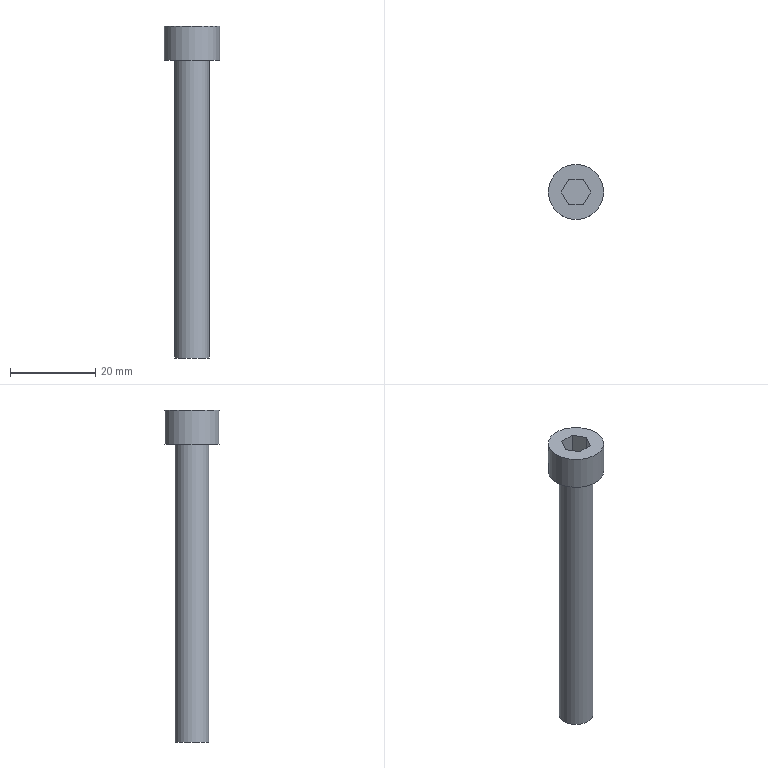Part | STEP file | 冲床-300配套压波_id198_x_t | 1 solid | 12 faces | box 13 x 13 x 78 mm | volume 4416 mm3 | plane 10 | cylinder 2 | commonest cylinder face diameters 8 x1 13 x1
STEP:
#1=CARTESIAN_POINT('',(1811.5,-85.,191.));
#2=VERTEX_POINT('',#1);
#3=CARTESIAN_POINT('',(1805.,-85.,191.));
#4=DIRECTION('',(0.,0.,1.));
#5=DIRECTION('',(1.,0.,0.));
#6=AXIS2_PLACEMENT_3D('',#3,#4,#5);
#7=CIRCLE('',#6,6.5);
#8=EDGE_CURVE('',#2,#2,#7,.T.);
#9=ORIENTED_EDGE('',*,*,#8,.T.);
#10=EDGE_LOOP('',(#9));
#11=FACE_BOUND('',#10,.T.);
#12=CARTESIAN_POINT('',(1803.268,-82.,191.));
#13=VERTEX_POINT('',#12);
#14=CARTESIAN_POINT('',(1806.732,-82.,191.));
#15=VERTEX_POINT('',#14);
#16=CARTESIAN_POINT('',(1803.268,-82.,191.));
#17=DIRECTION('',(1.,0.,0.));
#18=VECTOR('',#17,1.);
#19=LINE('',#16,#18);
#20=EDGE_CURVE('',#13,#15,#19,.T.);
#21=ORIENTED_EDGE('',*,*,#20,.T.);
#22=CARTESIAN_POINT('',(1808.464,-85.,191.));
#23=VERTEX_POINT('',#22);
#24=CARTESIAN_POINT('',(1806.732,-82.,191.));
#25=DIRECTION('',(0.5,-0.866,0.));
#26=VECTOR('',#25,1.);
#27=LINE('',#24,#26);
#28=EDGE_CURVE('',#15,#23,#27,.T.);
#29=ORIENTED_EDGE('',*,*,#28,.T.);
#30=CARTESIAN_POINT('',(1806.732,-88.,191.));
#31=VERTEX_POINT('',#30);
#32=CARTESIAN_POINT('',(1808.464,-85.,191.));
#33=DIRECTION('',(-0.5,-0.866,0.));
#34=VECTOR('',#33,1.);
#35=LINE('',#32,#34);
#36=EDGE_CURVE('',#23,#31,#35,.T.);
#37=ORIENTED_EDGE('',*,*,#36,.T.);
#38=CARTESIAN_POINT('',(1803.268,-88.,191.));
#39=VERTEX_POINT('',#38);
#40=CARTESIAN_POINT('',(1806.732,-88.,191.));
#41=DIRECTION('',(-1.,0.,0.));
#42=VECTOR('',#41,1.);
#43=LINE('',#40,#42);
#44=EDGE_CURVE('',#31,#39,#43,.T.);
#45=ORIENTED_EDGE('',*,*,#44,.T.);
#46=CARTESIAN_POINT('',(1801.536,-85.,191.));
#47=VERTEX_POINT('',#46);
#48=CARTESIAN_POINT('',(1803.268,-88.,191.));
#49=DIRECTION('',(-0.5,0.866,0.));
#50=VECTOR('',#49,1.);
#51=LINE('',#48,#50);
#52=EDGE_CURVE('',#39,#47,#51,.T.);
#53=ORIENTED_EDGE('',*,*,#52,.T.);
#54=CARTESIAN_POINT('',(1801.536,-85.,191.));
#55=DIRECTION('',(0.5,0.866,0.));
#56=VECTOR('',#55,1.);
#57=LINE('',#54,#56);
#58=EDGE_CURVE('',#47,#13,#57,.T.);
#59=ORIENTED_EDGE('',*,*,#58,.T.);
#60=EDGE_LOOP('',(#21,#29,#37,#45,#53,#59));
#61=FACE_BOUND('',#60,.T.);
#62=CARTESIAN_POINT('',(1811.5,-85.,191.));
#63=DIRECTION('',(0.,0.,-1.));
#64=DIRECTION('',(-1.,0.,0.));
#65=AXIS2_PLACEMENT_3D('',#62,#63,#64);
#66=PLANE('',#65);
#67=ADVANCED_FACE('',(#11,#61),#66,.F.);
#68=ORIENTED_EDGE('',*,*,#8,.F.);
#69=EDGE_LOOP('',(#68));
#70=FACE_BOUND('',#69,.T.);
#71=CARTESIAN_POINT('',(1811.5,-85.,183.));
#72=VERTEX_POINT('',#71);
#73=CARTESIAN_POINT('',(1805.,-85.,183.));
#74=DIRECTION('',(0.,0.,1.));
#75=DIRECTION('',(1.,0.,0.));
#76=AXIS2_PLACEMENT_3D('',#73,#74,#75);
#77=CIRCLE('',#76,6.5);
#78=EDGE_CURVE('',#72,#72,#77,.T.);
#79=ORIENTED_EDGE('',*,*,#78,.T.);
#80=EDGE_LOOP('',(#79));
#81=FACE_BOUND('',#80,.T.);
#82=CARTESIAN_POINT('',(1805.,-85.,184.1));
#83=DIRECTION('',(0.,0.,1.));
#84=DIRECTION('',(1.,0.,0.));
#85=AXIS2_PLACEMENT_3D('',#82,#83,#84);
#86=CYLINDRICAL_SURFACE('',#85,6.5);
#87=ADVANCED_FACE('',(#70,#81),#86,.T.);
#88=ORIENTED_EDGE('',*,*,#78,.F.);
#89=EDGE_LOOP('',(#88));
#90=FACE_BOUND('',#89,.T.);
#91=CARTESIAN_POINT('',(1809.,-85.,183.));
#92=VERTEX_POINT('',#91);
#93=CARTESIAN_POINT('',(1805.,-85.,183.));
#94=DIRECTION('',(0.,0.,1.));
#95=DIRECTION('',(1.,0.,0.));
#96=AXIS2_PLACEMENT_3D('',#93,#94,#95);
#97=CIRCLE('',#96,4.);
#98=EDGE_CURVE('',#92,#92,#97,.T.);
#99=ORIENTED_EDGE('',*,*,#98,.T.);
#100=EDGE_LOOP('',(#99));
#101=FACE_BOUND('',#100,.T.);
#102=CARTESIAN_POINT('',(1809.,-85.,183.));
#103=DIRECTION('',(0.,0.,1.));
#104=DIRECTION('',(1.,0.,0.));
#105=AXIS2_PLACEMENT_3D('',#102,#103,#104);
#106=PLANE('',#105);
#107=ADVANCED_FACE('',(#90,#101),#106,.F.);
#108=ORIENTED_EDGE('',*,*,#98,.F.);
#109=EDGE_LOOP('',(#108));
#110=FACE_BOUND('',#109,.T.);
#111=CARTESIAN_POINT('',(1809.,-85.,113.));
#112=VERTEX_POINT('',#111);
#113=CARTESIAN_POINT('',(1805.,-85.,113.));
#114=DIRECTION('',(0.,0.,1.));
#115=DIRECTION('',(1.,0.,0.));
#116=AXIS2_PLACEMENT_3D('',#113,#114,#115);
#117=CIRCLE('',#116,4.);
#118=EDGE_CURVE('',#112,#112,#117,.T.);
#119=ORIENTED_EDGE('',*,*,#118,.T.);
#120=EDGE_LOOP('',(#119));
#121=FACE_BOUND('',#120,.T.);
#122=CARTESIAN_POINT('',(1805.,-85.,184.1));
#123=DIRECTION('',(0.,0.,1.));
#124=DIRECTION('',(1.,0.,0.));
#125=AXIS2_PLACEMENT_3D('',#122,#123,#124);
#126=CYLINDRICAL_SURFACE('',#125,4.);
#127=ADVANCED_FACE('',(#110,#121),#126,.T.);
#128=ORIENTED_EDGE('',*,*,#118,.F.);
#129=EDGE_LOOP('',(#128));
#130=FACE_OUTER_BOUND('',#129,.T.);
#131=CARTESIAN_POINT('',(1805.,-85.,113.));
#132=DIRECTION('',(0.,0.,1.));
#133=DIRECTION('',(1.,0.,0.));
#134=AXIS2_PLACEMENT_3D('',#131,#132,#133);
#135=PLANE('',#134);
#136=ADVANCED_FACE('',(#130),#135,.F.);
#137=ORIENTED_EDGE('',*,*,#20,.F.);
#138=CARTESIAN_POINT('',(1803.268,-82.,185.72));
#139=VERTEX_POINT('',#138);
#140=CARTESIAN_POINT('',(1803.268,-82.,185.72));
#141=DIRECTION('',(0.,0.,-1.));
#142=VECTOR('',#141,1.);
#143=LINE('',#140,#142);
#144=EDGE_CURVE('',#13,#139,#143,.T.);
#145=ORIENTED_EDGE('',*,*,#144,.T.);
#146=CARTESIAN_POINT('',(1806.732,-82.,185.72));
#147=VERTEX_POINT('',#146);
#148=CARTESIAN_POINT('',(1803.268,-82.,185.72));
#149=DIRECTION('',(-1.,0.,0.));
#150=VECTOR('',#149,1.);
#151=LINE('',#148,#150);
#152=EDGE_CURVE('',#147,#139,#151,.T.);
#153=ORIENTED_EDGE('',*,*,#152,.F.);
#154=CARTESIAN_POINT('',(1806.732,-82.,185.72));
#155=DIRECTION('',(0.,0.,-1.));
#156=VECTOR('',#155,1.);
#157=LINE('',#154,#156);
#158=EDGE_CURVE('',#15,#147,#157,.T.);
#159=ORIENTED_EDGE('',*,*,#158,.F.);
#160=EDGE_LOOP('',(#137,#145,#153,#159));
#161=FACE_OUTER_BOUND('',#160,.T.);
#162=CARTESIAN_POINT('',(1803.268,-82.,185.72));
#163=DIRECTION('',(0.,-1.,0.));
#164=DIRECTION('',(1.,0.,0.));
#165=AXIS2_PLACEMENT_3D('',#162,#163,#164);
#166=PLANE('',#165);
#167=ADVANCED_FACE('',(#161),#166,.T.);
#168=ORIENTED_EDGE('',*,*,#28,.F.);
#169=ORIENTED_EDGE('',*,*,#158,.T.);
#170=CARTESIAN_POINT('',(1808.464,-85.,185.72));
#171=VERTEX_POINT('',#170);
#172=CARTESIAN_POINT('',(1806.732,-82.,185.72));
#173=DIRECTION('',(-0.5,0.866,0.));
#174=VECTOR('',#173,1.);
#175=LINE('',#172,#174);
#176=EDGE_CURVE('',#171,#147,#175,.T.);
#177=ORIENTED_EDGE('',*,*,#176,.F.);
#178=CARTESIAN_POINT('',(1808.464,-85.,185.72));
#179=DIRECTION('',(0.,0.,-1.));
#180=VECTOR('',#179,1.);
#181=LINE('',#178,#180);
#182=EDGE_CURVE('',#23,#171,#181,.T.);
#183=ORIENTED_EDGE('',*,*,#182,.F.);
#184=EDGE_LOOP('',(#168,#169,#177,#183));
#185=FACE_OUTER_BOUND('',#184,.T.);
#186=CARTESIAN_POINT('',(1806.732,-82.,185.72));
#187=DIRECTION('',(-0.866,-0.5,0.));
#188=DIRECTION('',(0.5,-0.866,0.));
#189=AXIS2_PLACEMENT_3D('',#186,#187,#188);
#190=PLANE('',#189);
#191=ADVANCED_FACE('',(#185),#190,.T.);
#192=ORIENTED_EDGE('',*,*,#36,.F.);
#193=ORIENTED_EDGE('',*,*,#182,.T.);
#194=CARTESIAN_POINT('',(1806.732,-88.,185.72));
#195=VERTEX_POINT('',#194);
#196=CARTESIAN_POINT('',(1808.464,-85.,185.72));
#197=DIRECTION('',(0.5,0.866,0.));
#198=VECTOR('',#197,1.);
#199=LINE('',#196,#198);
#200=EDGE_CURVE('',#195,#171,#199,.T.);
#201=ORIENTED_EDGE('',*,*,#200,.F.);
#202=CARTESIAN_POINT('',(1806.732,-88.,185.72));
#203=DIRECTION('',(0.,0.,-1.));
#204=VECTOR('',#203,1.);
#205=LINE('',#202,#204);
#206=EDGE_CURVE('',#31,#195,#205,.T.);
#207=ORIENTED_EDGE('',*,*,#206,.F.);
#208=EDGE_LOOP('',(#192,#193,#201,#207));
#209=FACE_OUTER_BOUND('',#208,.T.);
#210=CARTESIAN_POINT('',(1808.464,-85.,185.72));
#211=DIRECTION('',(-0.866,0.5,0.));
#212=DIRECTION('',(-0.5,-0.866,0.));
#213=AXIS2_PLACEMENT_3D('',#210,#211,#212);
#214=PLANE('',#213);
#215=ADVANCED_FACE('',(#209),#214,.T.);
#216=ORIENTED_EDGE('',*,*,#44,.F.);
#217=ORIENTED_EDGE('',*,*,#206,.T.);
#218=CARTESIAN_POINT('',(1803.268,-88.,185.72));
#219=VERTEX_POINT('',#218);
#220=CARTESIAN_POINT('',(1806.732,-88.,185.72));
#221=DIRECTION('',(1.,0.,0.));
#222=VECTOR('',#221,1.);
#223=LINE('',#220,#222);
#224=EDGE_CURVE('',#219,#195,#223,.T.);
#225=ORIENTED_EDGE('',*,*,#224,.F.);
#226=CARTESIAN_POINT('',(1803.268,-88.,185.72));
#227=DIRECTION('',(0.,0.,-1.));
#228=VECTOR('',#227,1.);
#229=LINE('',#226,#228);
#230=EDGE_CURVE('',#39,#219,#229,.T.);
#231=ORIENTED_EDGE('',*,*,#230,.F.);
#232=EDGE_LOOP('',(#216,#217,#225,#231));
#233=FACE_OUTER_BOUND('',#232,.T.);
#234=CARTESIAN_POINT('',(1806.732,-88.,185.72));
#235=DIRECTION('',(0.,1.,0.));
#236=DIRECTION('',(-1.,0.,0.));
#237=AXIS2_PLACEMENT_3D('',#234,#235,#236);
#238=PLANE('',#237);
#239=ADVANCED_FACE('',(#233),#238,.T.);
#240=ORIENTED_EDGE('',*,*,#52,.F.);
#241=ORIENTED_EDGE('',*,*,#230,.T.);
#242=CARTESIAN_POINT('',(1801.536,-85.,185.72));
#243=VERTEX_POINT('',#242);
#244=CARTESIAN_POINT('',(1803.268,-88.,185.72));
#245=DIRECTION('',(0.5,-0.866,0.));
#246=VECTOR('',#245,1.);
#247=LINE('',#244,#246);
#248=EDGE_CURVE('',#243,#219,#247,.T.);
#249=ORIENTED_EDGE('',*,*,#248,.F.);
#250=CARTESIAN_POINT('',(1801.536,-85.,185.72));
#251=DIRECTION('',(0.,0.,-1.));
#252=VECTOR('',#251,1.);
#253=LINE('',#250,#252);
#254=EDGE_CURVE('',#47,#243,#253,.T.);
#255=ORIENTED_EDGE('',*,*,#254,.F.);
#256=EDGE_LOOP('',(#240,#241,#249,#255));
#257=FACE_OUTER_BOUND('',#256,.T.);
#258=CARTESIAN_POINT('',(1803.268,-88.,185.72));
#259=DIRECTION('',(0.866,0.5,0.));
#260=DIRECTION('',(-0.5,0.866,0.));
#261=AXIS2_PLACEMENT_3D('',#258,#259,#260);
#262=PLANE('',#261);
#263=ADVANCED_FACE('',(#257),#262,.T.);
#264=ORIENTED_EDGE('',*,*,#58,.F.);
#265=ORIENTED_EDGE('',*,*,#254,.T.);
#266=CARTESIAN_POINT('',(1801.536,-85.,185.72));
#267=DIRECTION('',(-0.5,-0.866,0.));
#268=VECTOR('',#267,1.);
#269=LINE('',#266,#268);
#270=EDGE_CURVE('',#139,#243,#269,.T.);
#271=ORIENTED_EDGE('',*,*,#270,.F.);
#272=ORIENTED_EDGE('',*,*,#144,.F.);
#273=EDGE_LOOP('',(#264,#265,#271,#272));
#274=FACE_OUTER_BOUND('',#273,.T.);
#275=CARTESIAN_POINT('',(1801.536,-85.,185.72));
#276=DIRECTION('',(0.866,-0.5,0.));
#277=DIRECTION('',(0.5,0.866,0.));
#278=AXIS2_PLACEMENT_3D('',#275,#276,#277);
#279=PLANE('',#278);
#280=ADVANCED_FACE('',(#274),#279,.T.);
#281=ORIENTED_EDGE('',*,*,#152,.T.);
#282=ORIENTED_EDGE('',*,*,#270,.T.);
#283=ORIENTED_EDGE('',*,*,#248,.T.);
#284=ORIENTED_EDGE('',*,*,#224,.T.);
#285=ORIENTED_EDGE('',*,*,#200,.T.);
#286=ORIENTED_EDGE('',*,*,#176,.T.);
#287=EDGE_LOOP('',(#281,#282,#283,#284,#285,#286));
#288=FACE_OUTER_BOUND('',#287,.T.);
#289=CARTESIAN_POINT('',(1805.,-85.,185.72));
#290=DIRECTION('',(0.,0.,-1.));
#291=DIRECTION('',(-1.,0.,0.));
#292=AXIS2_PLACEMENT_3D('',#289,#290,#291);
#293=PLANE('',#292);
#294=ADVANCED_FACE('',(#288),#293,.F.);
#295=CLOSED_SHELL('',(#67,#87,#107,#127,#136,#167,#191,#215,#239,#263,#280,#294));
#296=MANIFOLD_SOLID_BREP('',#295);
#297=(LENGTH_UNIT()NAMED_UNIT(*)SI_UNIT(.MILLI.,.METRE.));
#298=UNCERTAINTY_MEASURE_WITH_UNIT(LENGTH_MEASURE(0.00002),#297,'','');
#299=(NAMED_UNIT(*)PLANE_ANGLE_UNIT()SI_UNIT($,.RADIAN.));
#300=PLANE_ANGLE_MEASURE_WITH_UNIT(PLANE_ANGLE_MEASURE(0.01745),#299);
#301=DIMENSIONAL_EXPONENTS(0.,0.,0.,0.,0.,0.,0.);
#302=(CONVERSION_BASED_UNIT('DEGREE',#300)NAMED_UNIT(#301)PLANE_ANGLE_UNIT());
#303=(NAMED_UNIT(*)SI_UNIT($,.STERADIAN.)SOLID_ANGLE_UNIT());
#304=(GEOMETRIC_REPRESENTATION_CONTEXT(3)GLOBAL_UNCERTAINTY_ASSIGNED_CONTEXT((#298))GLOBAL_UNIT_ASSIGNED_CONTEXT((#297,#302,#303))REPRESENTATION_CONTEXT('',''));
#305=ADVANCED_BREP_SHAPE_REPRESENTATION('',(#296),#304);